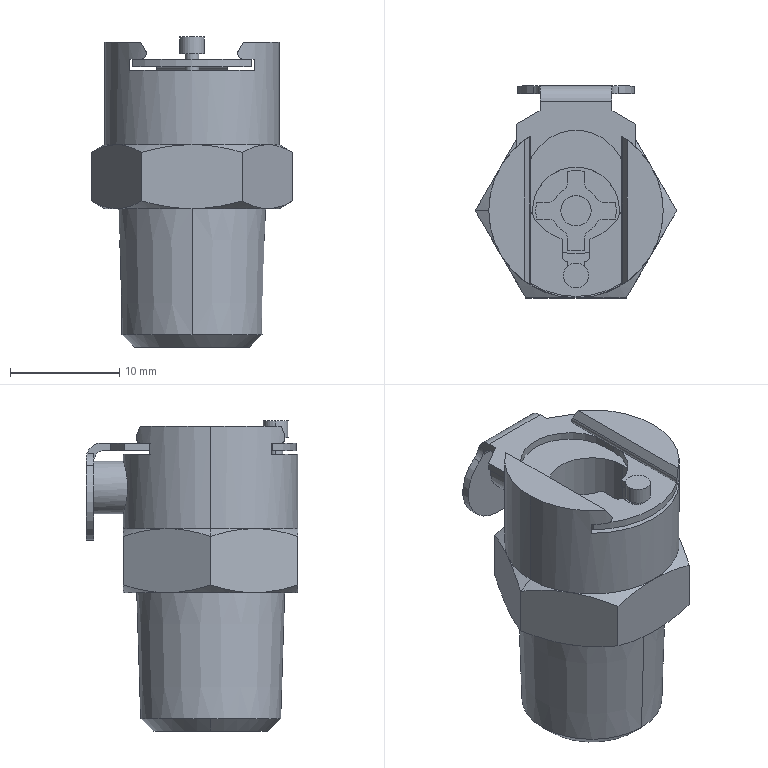Part | SolidWorks | 2 solids | 184 faces | box 18.478 x 19.431 x 28.448 mm | volume 3928 mm3 | plane 100 | cylinder 58 | cone 22 | spline 4 | commonest cylinder face diameters 1.524 x9 4.42 x8 7.366 x5 1.016 x4 2.845 x3 9.144 x3